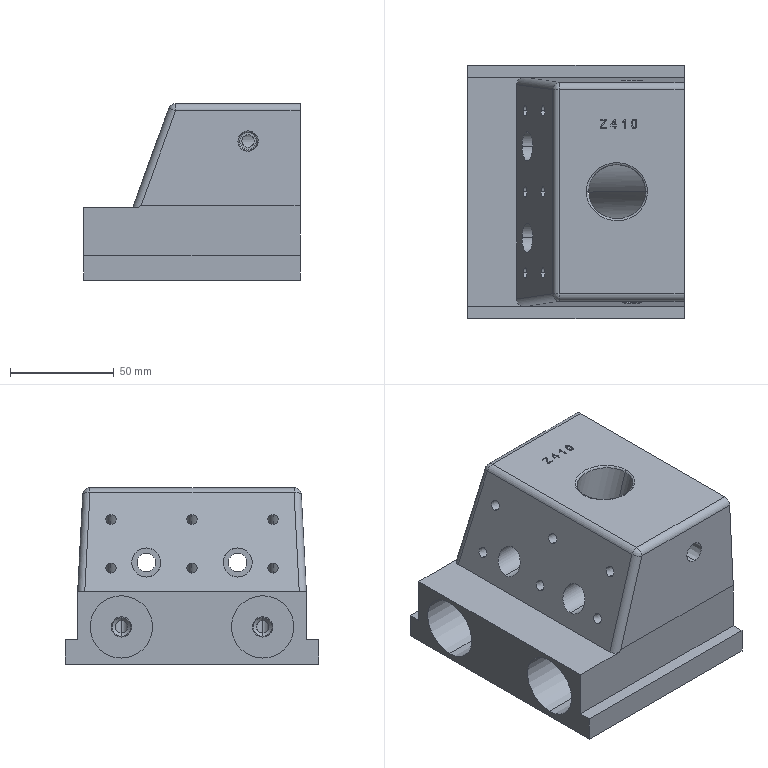Part | Creo | 1 solid | 205 faces | box 104 x 122 x 85 mm | volume 650533 mm3 | plane 64 | cylinder 60 | cone 38 | other 29 | sphere 10 | spline 4 | commonest cylinder face diameters 5 x12 6 x12 13 x8 7 x5 9 x4 10 x4